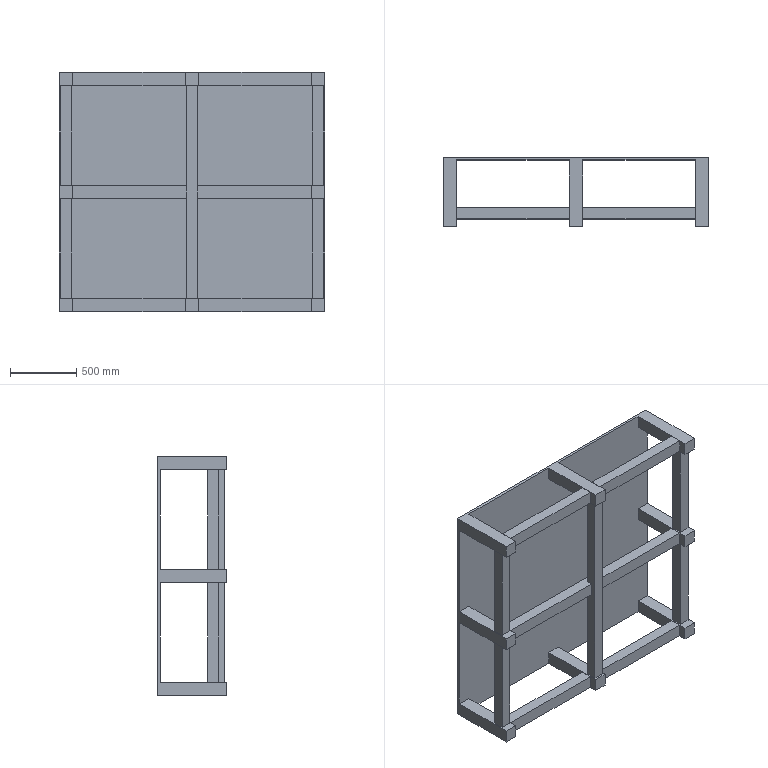Part | STEP file | 223_4 | 1 solid | 76 faces | box 2000 x 520 x 1800 mm | volume 184958483 mm3 | plane 76